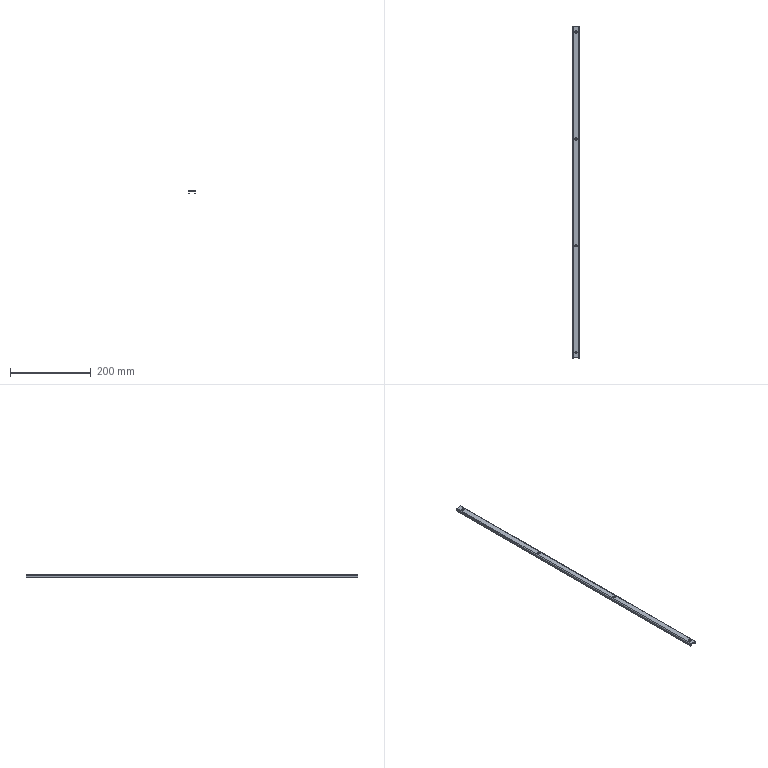Part | NX | features BREP 1 | 1 solid | 40 faces | box 17 x 820 x 7 mm | volume 42369 mm3 | plane 22 | cone 8 | cylinder 6 | torus 4 | commonest cylinder face diameters 0.2 x2 2 x2 4.2 x2
STEP:
#1=CARTESIAN_POINT('',(-2.7,395.,2.));
#2=VERTEX_POINT('',#1);
#3=CARTESIAN_POINT('',(2.7,395.,2.));
#4=VERTEX_POINT('',#3);
#5=CARTESIAN_POINT('',(0.,395.,2.));
#6=DIRECTION('',(0.,0.,1.));
#7=DIRECTION('',(1.,0.,0.));
#8=AXIS2_PLACEMENT_3D('',#5,#6,#7);
#9=CIRCLE('',#8,2.7);
#10=EDGE_CURVE('',#2,#4,#9,.T.);
#11=ORIENTED_EDGE('',*,*,#10,.T.);
#12=CARTESIAN_POINT('',(4.7,395.,0.));
#13=VERTEX_POINT('',#12);
#14=CARTESIAN_POINT('',(4.7,395.,0.));
#15=DIRECTION('',(0.7071,0.,-0.7071));
#16=VECTOR('',#15,1000.);
#17=LINE('',#14,#16);
#18=EDGE_CURVE('',#4,#13,#17,.T.);
#19=ORIENTED_EDGE('',*,*,#18,.T.);
#20=CARTESIAN_POINT('',(-4.7,395.,0.));
#21=VERTEX_POINT('',#20);
#22=CARTESIAN_POINT('',(0.,395.,0.));
#23=DIRECTION('',(0.,0.,-1.));
#24=DIRECTION('',(-1.,0.,0.));
#25=AXIS2_PLACEMENT_3D('',#22,#23,#24);
#26=CIRCLE('',#25,4.7);
#27=EDGE_CURVE('',#13,#21,#26,.T.);
#28=ORIENTED_EDGE('',*,*,#27,.T.);
#29=CARTESIAN_POINT('',(-4.7,395.,0.));
#30=DIRECTION('',(-0.7071,0.,-0.7071));
#31=VECTOR('',#30,1000.);
#32=LINE('',#29,#31);
#33=EDGE_CURVE('',#2,#21,#32,.T.);
#34=ORIENTED_EDGE('',*,*,#33,.F.);
#35=EDGE_LOOP('',(#11,#19,#28,#34));
#36=FACE_BOUND('',#35,.T.);
#37=CARTESIAN_POINT('',(0.,395.,0.));
#38=DIRECTION('',(0.,0.,-1.));
#39=DIRECTION('',(-1.,0.,0.));
#40=AXIS2_PLACEMENT_3D('',#37,#38,#39);
#41=CONICAL_SURFACE('',#40,4.7,0.7854);
#42=ADVANCED_FACE('',(#36),#41,.F.);
#43=CARTESIAN_POINT('',(-2.7,131.,2.));
#44=VERTEX_POINT('',#43);
#45=CARTESIAN_POINT('',(2.7,131.,2.));
#46=VERTEX_POINT('',#45);
#47=CARTESIAN_POINT('',(0.,131.,2.));
#48=DIRECTION('',(0.,0.,1.));
#49=DIRECTION('',(1.,0.,0.));
#50=AXIS2_PLACEMENT_3D('',#47,#48,#49);
#51=CIRCLE('',#50,2.7);
#52=EDGE_CURVE('',#44,#46,#51,.T.);
#53=ORIENTED_EDGE('',*,*,#52,.T.);
#54=CARTESIAN_POINT('',(4.7,131.,0.));
#55=VERTEX_POINT('',#54);
#56=CARTESIAN_POINT('',(4.7,131.,0.));
#57=DIRECTION('',(0.7071,0.,-0.7071));
#58=VECTOR('',#57,1000.);
#59=LINE('',#56,#58);
#60=EDGE_CURVE('',#46,#55,#59,.T.);
#61=ORIENTED_EDGE('',*,*,#60,.T.);
#62=CARTESIAN_POINT('',(-4.7,131.,0.));
#63=VERTEX_POINT('',#62);
#64=CARTESIAN_POINT('',(0.,131.,0.));
#65=DIRECTION('',(0.,0.,-1.));
#66=DIRECTION('',(-1.,0.,0.));
#67=AXIS2_PLACEMENT_3D('',#64,#65,#66);
#68=CIRCLE('',#67,4.7);
#69=EDGE_CURVE('',#55,#63,#68,.T.);
#70=ORIENTED_EDGE('',*,*,#69,.T.);
#71=CARTESIAN_POINT('',(-4.7,131.,0.));
#72=DIRECTION('',(-0.7071,0.,-0.7071));
#73=VECTOR('',#72,1000.);
#74=LINE('',#71,#73);
#75=EDGE_CURVE('',#44,#63,#74,.T.);
#76=ORIENTED_EDGE('',*,*,#75,.F.);
#77=EDGE_LOOP('',(#53,#61,#70,#76));
#78=FACE_BOUND('',#77,.T.);
#79=CARTESIAN_POINT('',(0.,131.,0.));
#80=DIRECTION('',(0.,0.,-1.));
#81=DIRECTION('',(-1.,0.,0.));
#82=AXIS2_PLACEMENT_3D('',#79,#80,#81);
#83=CONICAL_SURFACE('',#82,4.7,0.7854);
#84=ADVANCED_FACE('',(#78),#83,.F.);
#85=CARTESIAN_POINT('',(-2.7,-133.,2.));
#86=VERTEX_POINT('',#85);
#87=CARTESIAN_POINT('',(2.7,-133.,2.));
#88=VERTEX_POINT('',#87);
#89=CARTESIAN_POINT('',(0.,-133.,2.));
#90=DIRECTION('',(0.,0.,1.));
#91=DIRECTION('',(1.,0.,0.));
#92=AXIS2_PLACEMENT_3D('',#89,#90,#91);
#93=CIRCLE('',#92,2.7);
#94=EDGE_CURVE('',#86,#88,#93,.T.);
#95=ORIENTED_EDGE('',*,*,#94,.T.);
#96=CARTESIAN_POINT('',(4.7,-133.,0.));
#97=VERTEX_POINT('',#96);
#98=CARTESIAN_POINT('',(4.7,-133.,0.));
#99=DIRECTION('',(0.7071,0.,-0.7071));
#100=VECTOR('',#99,1000.);
#101=LINE('',#98,#100);
#102=EDGE_CURVE('',#88,#97,#101,.T.);
#103=ORIENTED_EDGE('',*,*,#102,.T.);
#104=CARTESIAN_POINT('',(-4.7,-133.,0.));
#105=VERTEX_POINT('',#104);
#106=CARTESIAN_POINT('',(0.,-133.,0.));
#107=DIRECTION('',(0.,0.,-1.));
#108=DIRECTION('',(-1.,0.,0.));
#109=AXIS2_PLACEMENT_3D('',#106,#107,#108);
#110=CIRCLE('',#109,4.7);
#111=EDGE_CURVE('',#97,#105,#110,.T.);
#112=ORIENTED_EDGE('',*,*,#111,.T.);
#113=CARTESIAN_POINT('',(-4.7,-133.,0.));
#114=DIRECTION('',(-0.7071,0.,-0.7071));
#115=VECTOR('',#114,1000.);
#116=LINE('',#113,#115);
#117=EDGE_CURVE('',#86,#105,#116,.T.);
#118=ORIENTED_EDGE('',*,*,#117,.F.);
#119=EDGE_LOOP('',(#95,#103,#112,#118));
#120=FACE_BOUND('',#119,.T.);
#121=CARTESIAN_POINT('',(0.,-133.,0.));
#122=DIRECTION('',(0.,0.,-1.));
#123=DIRECTION('',(-1.,0.,0.));
#124=AXIS2_PLACEMENT_3D('',#121,#122,#123);
#125=CONICAL_SURFACE('',#124,4.7,0.7854);
#126=ADVANCED_FACE('',(#120),#125,.F.);
#127=CARTESIAN_POINT('',(-2.7,-397.,2.));
#128=VERTEX_POINT('',#127);
#129=CARTESIAN_POINT('',(2.7,-397.,2.));
#130=VERTEX_POINT('',#129);
#131=CARTESIAN_POINT('',(0.,-397.,2.));
#132=DIRECTION('',(0.,0.,1.));
#133=DIRECTION('',(1.,0.,0.));
#134=AXIS2_PLACEMENT_3D('',#131,#132,#133);
#135=CIRCLE('',#134,2.7);
#136=EDGE_CURVE('',#128,#130,#135,.T.);
#137=ORIENTED_EDGE('',*,*,#136,.T.);
#138=CARTESIAN_POINT('',(4.7,-397.,0.));
#139=VERTEX_POINT('',#138);
#140=CARTESIAN_POINT('',(4.7,-397.,0.));
#141=DIRECTION('',(0.7071,0.,-0.7071));
#142=VECTOR('',#141,1000.);
#143=LINE('',#140,#142);
#144=EDGE_CURVE('',#130,#139,#143,.T.);
#145=ORIENTED_EDGE('',*,*,#144,.T.);
#146=CARTESIAN_POINT('',(-4.7,-397.,0.));
#147=VERTEX_POINT('',#146);
#148=CARTESIAN_POINT('',(0.,-397.,0.));
#149=DIRECTION('',(0.,0.,-1.));
#150=DIRECTION('',(-1.,0.,0.));
#151=AXIS2_PLACEMENT_3D('',#148,#149,#150);
#152=CIRCLE('',#151,4.7);
#153=EDGE_CURVE('',#139,#147,#152,.T.);
#154=ORIENTED_EDGE('',*,*,#153,.T.);
#155=CARTESIAN_POINT('',(-4.7,-397.,0.));
#156=DIRECTION('',(-0.7071,0.,-0.7071));
#157=VECTOR('',#156,1000.);
#158=LINE('',#155,#157);
#159=EDGE_CURVE('',#128,#147,#158,.T.);
#160=ORIENTED_EDGE('',*,*,#159,.F.);
#161=EDGE_LOOP('',(#137,#145,#154,#160));
#162=FACE_BOUND('',#161,.T.);
#163=CARTESIAN_POINT('',(0.,-397.,0.));
#164=DIRECTION('',(0.,0.,-1.));
#165=DIRECTION('',(-1.,0.,0.));
#166=AXIS2_PLACEMENT_3D('',#163,#164,#165);
#167=CONICAL_SURFACE('',#166,4.7,0.7854);
#168=ADVANCED_FACE('',(#162),#167,.F.);
#169=CARTESIAN_POINT('',(6.4,-410.,2.));
#170=VERTEX_POINT('',#169);
#171=CARTESIAN_POINT('',(-6.4,-410.,2.));
#172=VERTEX_POINT('',#171);
#173=CARTESIAN_POINT('',(-6.5,-410.,2.));
#174=DIRECTION('',(-1.,0.,0.));
#175=VECTOR('',#174,1000.);
#176=LINE('',#173,#175);
#177=EDGE_CURVE('',#170,#172,#176,.T.);
#178=ORIENTED_EDGE('',*,*,#177,.F.);
#179=CARTESIAN_POINT('',(6.4,410.,2.));
#180=VERTEX_POINT('',#179);
#181=CARTESIAN_POINT('',(6.4,410.,2.));
#182=DIRECTION('',(0.,-1.,0.));
#183=VECTOR('',#182,1000.);
#184=LINE('',#181,#183);
#185=EDGE_CURVE('',#180,#170,#184,.T.);
#186=ORIENTED_EDGE('',*,*,#185,.F.);
#187=CARTESIAN_POINT('',(-6.4,410.,2.));
#188=VERTEX_POINT('',#187);
#189=CARTESIAN_POINT('',(-6.5,410.,2.));
#190=DIRECTION('',(-1.,0.,0.));
#191=VECTOR('',#190,1000.);
#192=LINE('',#189,#191);
#193=EDGE_CURVE('',#180,#188,#192,.T.);
#194=ORIENTED_EDGE('',*,*,#193,.T.);
#195=CARTESIAN_POINT('',(-6.4,410.,2.));
#196=DIRECTION('',(0.,-1.,0.));
#197=VECTOR('',#196,1000.);
#198=LINE('',#195,#197);
#199=EDGE_CURVE('',#188,#172,#198,.T.);
#200=ORIENTED_EDGE('',*,*,#199,.T.);
#201=EDGE_LOOP('',(#178,#186,#194,#200));
#202=FACE_BOUND('',#201,.T.);
#203=ORIENTED_EDGE('',*,*,#10,.F.);
#204=CARTESIAN_POINT('',(0.,395.,2.));
#205=DIRECTION('',(0.,0.,1.));
#206=DIRECTION('',(1.,0.,0.));
#207=AXIS2_PLACEMENT_3D('',#204,#205,#206);
#208=CIRCLE('',#207,2.7);
#209=EDGE_CURVE('',#4,#2,#208,.T.);
#210=ORIENTED_EDGE('',*,*,#209,.F.);
#211=EDGE_LOOP('',(#203,#210));
#212=FACE_BOUND('',#211,.T.);
#213=ORIENTED_EDGE('',*,*,#136,.F.);
#214=CARTESIAN_POINT('',(0.,-397.,2.));
#215=DIRECTION('',(0.,0.,1.));
#216=DIRECTION('',(1.,0.,0.));
#217=AXIS2_PLACEMENT_3D('',#214,#215,#216);
#218=CIRCLE('',#217,2.7);
#219=EDGE_CURVE('',#130,#128,#218,.T.);
#220=ORIENTED_EDGE('',*,*,#219,.F.);
#221=EDGE_LOOP('',(#213,#220));
#222=FACE_BOUND('',#221,.T.);
#223=ORIENTED_EDGE('',*,*,#94,.F.);
#224=CARTESIAN_POINT('',(0.,-133.,2.));
#225=DIRECTION('',(0.,0.,1.));
#226=DIRECTION('',(1.,0.,0.));
#227=AXIS2_PLACEMENT_3D('',#224,#225,#226);
#228=CIRCLE('',#227,2.7);
#229=EDGE_CURVE('',#88,#86,#228,.T.);
#230=ORIENTED_EDGE('',*,*,#229,.F.);
#231=EDGE_LOOP('',(#223,#230));
#232=FACE_BOUND('',#231,.T.);
#233=ORIENTED_EDGE('',*,*,#52,.F.);
#234=CARTESIAN_POINT('',(0.,131.,2.));
#235=DIRECTION('',(0.,0.,1.));
#236=DIRECTION('',(1.,0.,0.));
#237=AXIS2_PLACEMENT_3D('',#234,#235,#236);
#238=CIRCLE('',#237,2.7);
#239=EDGE_CURVE('',#46,#44,#238,.T.);
#240=ORIENTED_EDGE('',*,*,#239,.F.);
#241=EDGE_LOOP('',(#233,#240));
#242=FACE_BOUND('',#241,.T.);
#243=CARTESIAN_POINT('',(-6.5,410.,2.));
#244=DIRECTION('',(0.,0.,1.));
#245=DIRECTION('',(1.,0.,0.));
#246=AXIS2_PLACEMENT_3D('',#243,#244,#245);
#247=PLANE('',#246);
#248=ADVANCED_FACE('',(#202,#212,#222,#232,#242),#247,.T.);
#249=CARTESIAN_POINT('',(7.5,410.,-0.1));
#250=VERTEX_POINT('',#249);
#251=CARTESIAN_POINT('',(8.5,410.,-0.1));
#252=VERTEX_POINT('',#251);
#253=CARTESIAN_POINT('',(6.5,410.,-0.1));
#254=DIRECTION('',(1.,0.,0.));
#255=VECTOR('',#254,1000.);
#256=LINE('',#253,#255);
#257=EDGE_CURVE('',#250,#252,#256,.T.);
#258=ORIENTED_EDGE('',*,*,#257,.F.);
#259=CARTESIAN_POINT('',(6.4,410.,1.));
#260=VERTEX_POINT('',#259);
#261=CARTESIAN_POINT('',(6.4,410.,-0.1));
#262=DIRECTION('',(0.,-1.,0.));
#263=DIRECTION('',(0.,0.,1.));
#264=AXIS2_PLACEMENT_3D('',#261,#262,#263);
#265=CIRCLE('',#264,1.1);
#266=EDGE_CURVE('',#250,#260,#265,.T.);
#267=ORIENTED_EDGE('',*,*,#266,.T.);
#268=CARTESIAN_POINT('',(6.4,410.,2.));
#269=DIRECTION('',(0.,0.,-1.));
#270=VECTOR('',#269,1000.);
#271=LINE('',#268,#270);
#272=EDGE_CURVE('',#180,#260,#271,.T.);
#273=ORIENTED_EDGE('',*,*,#272,.F.);
#274=CARTESIAN_POINT('',(6.4,410.,-0.1));
#275=DIRECTION('',(0.,-1.,0.));
#276=DIRECTION('',(1.,0.,0.));
#277=AXIS2_PLACEMENT_3D('',#274,#275,#276);
#278=CIRCLE('',#277,2.1);
#279=EDGE_CURVE('',#252,#180,#278,.T.);
#280=ORIENTED_EDGE('',*,*,#279,.F.);
#281=EDGE_LOOP('',(#258,#267,#273,#280));
#282=FACE_BOUND('',#281,.T.);
#283=CARTESIAN_POINT('',(6.5,410.,-0.1));
#284=DIRECTION('',(0.,1.,0.));
#285=DIRECTION('',(1.,0.,0.));
#286=AXIS2_PLACEMENT_3D('',#283,#284,#285);
#287=PLANE('',#286);
#288=ADVANCED_FACE('',(#282),#287,.T.);
#289=CARTESIAN_POINT('',(8.5,410.,-4.));
#290=VERTEX_POINT('',#289);
#291=CARTESIAN_POINT('',(8.5,410.,0.));
#292=DIRECTION('',(0.,0.,1.));
#293=VECTOR('',#292,1000.);
#294=LINE('',#291,#293);
#295=EDGE_CURVE('',#290,#252,#294,.T.);
#296=ORIENTED_EDGE('',*,*,#295,.F.);
#297=CARTESIAN_POINT('',(6.5,410.,-4.));
#298=VERTEX_POINT('',#297);
#299=CARTESIAN_POINT('',(6.4,410.,-4.));
#300=DIRECTION('',(-1.,0.,0.));
#301=VECTOR('',#300,1000.);
#302=LINE('',#299,#301);
#303=EDGE_CURVE('',#290,#298,#302,.T.);
#304=ORIENTED_EDGE('',*,*,#303,.T.);
#305=CARTESIAN_POINT('',(6.5,410.,-1.195));
#306=VERTEX_POINT('',#305);
#307=CARTESIAN_POINT('',(6.5,410.,0.));
#308=DIRECTION('',(0.,0.,1.));
#309=VECTOR('',#308,1000.);
#310=LINE('',#307,#309);
#311=EDGE_CURVE('',#298,#306,#310,.T.);
#312=ORIENTED_EDGE('',*,*,#311,.T.);
#313=CARTESIAN_POINT('',(6.4,410.,-0.1));
#314=DIRECTION('',(0.,-1.,0.));
#315=DIRECTION('',(0.,0.,1.));
#316=AXIS2_PLACEMENT_3D('',#313,#314,#315);
#317=CIRCLE('',#316,1.1);
#318=EDGE_CURVE('',#306,#250,#317,.T.);
#319=ORIENTED_EDGE('',*,*,#318,.T.);
#320=ORIENTED_EDGE('',*,*,#257,.T.);
#321=EDGE_LOOP('',(#296,#304,#312,#319,#320));
#322=FACE_BOUND('',#321,.T.);
#323=CARTESIAN_POINT('',(6.4,410.,2.));
#324=DIRECTION('',(0.,1.,0.));
#325=DIRECTION('',(1.,0.,0.));
#326=AXIS2_PLACEMENT_3D('',#323,#324,#325);
#327=PLANE('',#326);
#328=ADVANCED_FACE('',(#322),#327,.T.);
#329=CARTESIAN_POINT('',(6.4,-410.,1.));
#330=VERTEX_POINT('',#329);
#331=CARTESIAN_POINT('',(6.4,-410.,0.));
#332=DIRECTION('',(0.,0.,1.));
#333=VECTOR('',#332,1000.);
#334=LINE('',#331,#333);
#335=EDGE_CURVE('',#330,#170,#334,.T.);
#336=ORIENTED_EDGE('',*,*,#335,.F.);
#337=CARTESIAN_POINT('',(7.5,-410.,-0.1));
#338=VERTEX_POINT('',#337);
#339=CARTESIAN_POINT('',(6.4,-410.,-0.1));
#340=DIRECTION('',(0.,1.,0.));
#341=DIRECTION('',(0.,0.,-1.));
#342=AXIS2_PLACEMENT_3D('',#339,#340,#341);
#343=CIRCLE('',#342,1.1);
#344=EDGE_CURVE('',#330,#338,#343,.T.);
#345=ORIENTED_EDGE('',*,*,#344,.T.);
#346=CARTESIAN_POINT('',(8.5,-410.,-0.1));
#347=VERTEX_POINT('',#346);
#348=CARTESIAN_POINT('',(8.5,-410.,-0.1));
#349=DIRECTION('',(-1.,0.,0.));
#350=VECTOR('',#349,1000.);
#351=LINE('',#348,#350);
#352=EDGE_CURVE('',#347,#338,#351,.T.);
#353=ORIENTED_EDGE('',*,*,#352,.F.);
#354=CARTESIAN_POINT('',(6.4,-410.,-0.1));
#355=DIRECTION('',(0.,-1.,0.));
#356=DIRECTION('',(1.,0.,0.));
#357=AXIS2_PLACEMENT_3D('',#354,#355,#356);
#358=CIRCLE('',#357,2.1);
#359=EDGE_CURVE('',#347,#170,#358,.T.);
#360=ORIENTED_EDGE('',*,*,#359,.T.);
#361=EDGE_LOOP('',(#336,#345,#353,#360));
#362=FACE_BOUND('',#361,.T.);
#363=CARTESIAN_POINT('',(6.4,-410.,0.));
#364=DIRECTION('',(0.,-1.,0.));
#365=DIRECTION('',(0.,0.,-1.));
#366=AXIS2_PLACEMENT_3D('',#363,#364,#365);
#367=PLANE('',#366);
#368=ADVANCED_FACE('',(#362),#367,.T.);
#369=CARTESIAN_POINT('',(-6.4,-410.,1.));
#370=VERTEX_POINT('',#369);
#371=CARTESIAN_POINT('',(-6.4,-410.,2.));
#372=DIRECTION('',(0.,0.,-1.));
#373=VECTOR('',#372,1000.);
#374=LINE('',#371,#373);
#375=EDGE_CURVE('',#172,#370,#374,.T.);
#376=ORIENTED_EDGE('',*,*,#375,.T.);
#377=CARTESIAN_POINT('',(6.4,-410.,1.));
#378=DIRECTION('',(1.,0.,0.));
#379=VECTOR('',#378,1000.);
#380=LINE('',#377,#379);
#381=EDGE_CURVE('',#370,#330,#380,.T.);
#382=ORIENTED_EDGE('',*,*,#381,.T.);
#383=ORIENTED_EDGE('',*,*,#335,.T.);
#384=ORIENTED_EDGE('',*,*,#177,.T.);
#385=EDGE_LOOP('',(#376,#382,#383,#384));
#386=FACE_BOUND('',#385,.T.);
#387=CARTESIAN_POINT('',(8.5,-410.,-0.1));
#388=DIRECTION('',(0.,-1.,0.));
#389=DIRECTION('',(0.,0.,-1.));
#390=AXIS2_PLACEMENT_3D('',#387,#388,#389);
#391=PLANE('',#390);
#392=ADVANCED_FACE('',(#386),#391,.T.);
#393=CARTESIAN_POINT('',(-6.4,410.,1.));
#394=VERTEX_POINT('',#393);
#395=CARTESIAN_POINT('',(-6.4,410.,0.));
#396=DIRECTION('',(0.,0.,1.));
#397=VECTOR('',#396,1000.);
#398=LINE('',#395,#397);
#399=EDGE_CURVE('',#394,#188,#398,.T.);
#400=ORIENTED_EDGE('',*,*,#399,.F.);
#401=CARTESIAN_POINT('',(-7.5,410.,-0.1));
#402=VERTEX_POINT('',#401);
#403=CARTESIAN_POINT('',(-6.4,410.,-0.1));
#404=DIRECTION('',(0.,-1.,0.));
#405=DIRECTION('',(0.,0.,1.));
#406=AXIS2_PLACEMENT_3D('',#403,#404,#405);
#407=CIRCLE('',#406,1.1);
#408=EDGE_CURVE('',#394,#402,#407,.T.);
#409=ORIENTED_EDGE('',*,*,#408,.T.);
#410=CARTESIAN_POINT('',(-8.5,410.,-0.1));
#411=VERTEX_POINT('',#410);
#412=CARTESIAN_POINT('',(-8.5,410.,-0.1));
#413=DIRECTION('',(1.,0.,0.));
#414=VECTOR('',#413,1000.);
#415=LINE('',#412,#414);
#416=EDGE_CURVE('',#411,#402,#415,.T.);
#417=ORIENTED_EDGE('',*,*,#416,.F.);
#418=CARTESIAN_POINT('',(-6.4,410.,-0.1));
#419=DIRECTION('',(0.,-1.,0.));
#420=DIRECTION('',(1.,0.,0.));
#421=AXIS2_PLACEMENT_3D('',#418,#419,#420);
#422=CIRCLE('',#421,2.1);
#423=EDGE_CURVE('',#188,#411,#422,.T.);
#424=ORIENTED_EDGE('',*,*,#423,.F.);
#425=EDGE_LOOP('',(#400,#409,#417,#424));
#426=FACE_BOUND('',#425,.T.);
#427=CARTESIAN_POINT('',(-6.4,410.,0.));
#428=DIRECTION('',(0.,1.,0.));
#429=DIRECTION('',(1.,0.,0.));
#430=AXIS2_PLACEMENT_3D('',#427,#428,#429);
#431=PLANE('',#430);
#432=ADVANCED_FACE('',(#426),#431,.T.);
#433=ORIENTED_EDGE('',*,*,#272,.T.);
#434=CARTESIAN_POINT('',(-6.4,410.,1.));
#435=DIRECTION('',(-1.,0.,0.));
#436=VECTOR('',#435,1000.);
#437=LINE('',#434,#436);
#438=EDGE_CURVE('',#260,#394,#437,.T.);
#439=ORIENTED_EDGE('',*,*,#438,.T.);
#440=ORIENTED_EDGE('',*,*,#399,.T.);
#441=ORIENTED_EDGE('',*,*,#193,.F.);
#442=EDGE_LOOP('',(#433,#439,#440,#441));
#443=FACE_BOUND('',#442,.T.);
#444=CARTESIAN_POINT('',(-8.5,410.,-0.1));
#445=DIRECTION('',(0.,1.,0.));
#446=DIRECTION('',(1.,0.,0.));
#447=AXIS2_PLACEMENT_3D('',#444,#445,#446);
#448=PLANE('',#447);
#449=ADVANCED_FACE('',(#443),#448,.T.);
#450=CARTESIAN_POINT('',(-7.5,-410.,-0.1));
#451=VERTEX_POINT('',#450);
#452=CARTESIAN_POINT('',(-8.5,-410.,-0.1));
#453=VERTEX_POINT('',#452);
#454=CARTESIAN_POINT('',(-6.5,-410.,-0.1));
#455=DIRECTION('',(-1.,0.,0.));
#456=VECTOR('',#455,1000.);
#457=LINE('',#454,#456);
#458=EDGE_CURVE('',#451,#453,#457,.T.);
#459=ORIENTED_EDGE('',*,*,#458,.F.);
#460=CARTESIAN_POINT('',(-6.4,-410.,-0.1));
#461=DIRECTION('',(0.,1.,0.));
#462=DIRECTION('',(0.,0.,-1.));
#463=AXIS2_PLACEMENT_3D('',#460,#461,#462);
#464=CIRCLE('',#463,1.1);
#465=EDGE_CURVE('',#451,#370,#464,.T.);
#466=ORIENTED_EDGE('',*,*,#465,.T.);
#467=ORIENTED_EDGE('',*,*,#375,.F.);
#468=CARTESIAN_POINT('',(-6.4,-410.,-0.1));
#469=DIRECTION('',(0.,-1.,0.));
#470=DIRECTION('',(1.,0.,0.));
#471=AXIS2_PLACEMENT_3D('',#468,#469,#470);
#472=CIRCLE('',#471,2.1);
#473=EDGE_CURVE('',#172,#453,#472,.T.);
#474=ORIENTED_EDGE('',*,*,#473,.T.);
#475=EDGE_LOOP('',(#459,#466,#467,#474));
#476=FACE_BOUND('',#475,.T.);
#477=CARTESIAN_POINT('',(-6.5,-410.,-0.1));
#478=DIRECTION('',(0.,-1.,0.));
#479=DIRECTION('',(0.,0.,-1.));
#480=AXIS2_PLACEMENT_3D('',#477,#478,#479);
#481=PLANE('',#480);
#482=ADVANCED_FACE('',(#476),#481,.T.);
#483=CARTESIAN_POINT('',(-8.5,-410.,-4.));
#484=VERTEX_POINT('',#483);
#485=CARTESIAN_POINT('',(-8.5,-410.,0.));
#486=DIRECTION('',(0.,0.,-1.));
#487=VECTOR('',#486,1000.);
#488=LINE('',#485,#487);
#489=EDGE_CURVE('',#453,#484,#488,.T.);
#490=ORIENTED_EDGE('',*,*,#489,.T.);
#491=CARTESIAN_POINT('',(-6.5,-410.,-4.));
#492=VERTEX_POINT('',#491);
#493=CARTESIAN_POINT('',(-6.4,-410.,-4.));
#494=DIRECTION('',(1.,0.,0.));
#495=VECTOR('',#494,1000.);
#496=LINE('',#493,#495);
#497=EDGE_CURVE('',#484,#492,#496,.T.);
#498=ORIENTED_EDGE('',*,*,#497,.T.);
#499=CARTESIAN_POINT('',(-6.5,-410.,-1.195));
#500=VERTEX_POINT('',#499);
#501=CARTESIAN_POINT('',(-6.5,-410.,0.));
#502=DIRECTION('',(0.,0.,-1.));
#503=VECTOR('',#502,1000.);
#504=LINE('',#501,#503);
#505=EDGE_CURVE('',#500,#492,#504,.T.);
#506=ORIENTED_EDGE('',*,*,#505,.F.);
#507=CARTESIAN_POINT('',(-6.4,-410.,-0.1));
#508=DIRECTION('',(0.,1.,0.));
#509=DIRECTION('',(0.,0.,-1.));
#510=AXIS2_PLACEMENT_3D('',#507,#508,#509);
#511=CIRCLE('',#510,1.1);
#512=EDGE_CURVE('',#500,#451,#511,.T.);
#513=ORIENTED_EDGE('',*,*,#512,.T.);
#514=ORIENTED_EDGE('',*,*,#458,.T.);
#515=EDGE_LOOP('',(#490,#498,#506,#513,#514));
#516=FACE_BOUND('',#515,.T.);
#517=CARTESIAN_POINT('',(-6.4,-410.,2.));
#518=DIRECTION('',(0.,-1.,0.));
#519=DIRECTION('',(0.,0.,-1.));
#520=AXIS2_PLACEMENT_3D('',#517,#518,#519);
#521=PLANE('',#520);
#522=ADVANCED_FACE('',(#516),#521,.T.);
#523=CARTESIAN_POINT('',(-6.5,409.,-5.));
#524=VERTEX_POINT('',#523);
#525=CARTESIAN_POINT('',(-6.5,-409.,-5.));
#526=VERTEX_POINT('',#525);
#527=CARTESIAN_POINT('',(-6.5,410.,-5.));
#528=DIRECTION('',(0.,-1.,0.));
#529=VECTOR('',#528,1000.);
#530=LINE('',#527,#529);
#531=EDGE_CURVE('',#524,#526,#530,.T.);
#532=ORIENTED_EDGE('',*,*,#531,.F.);
#533=CARTESIAN_POINT('',(-6.5,410.,-4.));
#534=VERTEX_POINT('',#533);
#535=CARTESIAN_POINT('',(-6.5,409.,-5.));
#536=DIRECTION('',(0.,0.7071,0.7071));
#537=VECTOR('',#536,1000.);
#538=LINE('',#535,#537);
#539=EDGE_CURVE('',#524,#534,#538,.T.);
#540=ORIENTED_EDGE('',*,*,#539,.T.);
#541=CARTESIAN_POINT('',(-6.5,410.,-1.195));
#542=VERTEX_POINT('',#541);
#543=CARTESIAN_POINT('',(-6.5,410.,0.));
#544=DIRECTION('',(0.,0.,-1.));
#545=VECTOR('',#544,1000.);
#546=LINE('',#543,#545);
#547=EDGE_CURVE('',#542,#534,#546,.T.);
#548=ORIENTED_EDGE('',*,*,#547,.F.);
#549=CARTESIAN_POINT('',(-6.5,409.,-0.1));
#550=VERTEX_POINT('',#549);
#551=CARTESIAN_POINT('',(-6.5,410.,-1.195));
#552=CARTESIAN_POINT('',(-6.5,410.,-0.9262));
#553=CARTESIAN_POINT('',(-6.5,409.841,-0.5362));
#554=CARTESIAN_POINT('',(-6.5,409.369,-0.219));
#555=CARTESIAN_POINT('',(-6.5,409.163,-0.1517));
#556=CARTESIAN_POINT('',(-6.5,409.,-0.1));
#557=B_SPLINE_CURVE_WITH_KNOTS('',3,(#551,#552,#553,#554,#555,#556),.UNSPECIFIED.,.F.,.F.,(4,1,1,4),(0.,0.5,0.75,1.),.UNSPECIFIED.);
#558=EDGE_CURVE('',#542,#550,#557,.T.);
#559=ORIENTED_EDGE('',*,*,#558,.T.);
#560=CARTESIAN_POINT('',(-6.5,-409.,-0.1));
#561=VERTEX_POINT('',#560);
#562=CARTESIAN_POINT('',(-6.5,410.,-0.1));
#563=DIRECTION('',(0.,-1.,0.));
#564=VECTOR('',#563,1000.);
#565=LINE('',#562,#564);
#566=EDGE_CURVE('',#550,#561,#565,.T.);
#567=ORIENTED_EDGE('',*,*,#566,.T.);
#568=CARTESIAN_POINT('',(-6.5,-409.,-0.1));
#569=CARTESIAN_POINT('',(-6.5,-409.162,-0.1513));
#570=CARTESIAN_POINT('',(-6.5,-409.369,-0.2191));
#571=CARTESIAN_POINT('',(-6.5,-409.84,-0.5364));
#572=CARTESIAN_POINT('',(-6.5,-410.,-0.9248));
#573=CARTESIAN_POINT('',(-6.5,-410.,-1.195));
#574=B_SPLINE_CURVE_WITH_KNOTS('',3,(#568,#569,#570,#571,#572,#573),.UNSPECIFIED.,.F.,.F.,(4,1,1,4),(0.,0.25,0.5,1.),.UNSPECIFIED.);
#575=EDGE_CURVE('',#561,#500,#574,.T.);
#576=ORIENTED_EDGE('',*,*,#575,.T.);
#577=ORIENTED_EDGE('',*,*,#505,.T.);
#578=CARTESIAN_POINT('',(-6.5,-410.,-4.));
#579=DIRECTION('',(0.,0.7071,-0.7071));
#580=VECTOR('',#579,1000.);
#581=LINE('',#578,#580);
#582=EDGE_CURVE('',#492,#526,#581,.T.);
#583=ORIENTED_EDGE('',*,*,#582,.T.);
#584=EDGE_LOOP('',(#532,#540,#548,#559,#567,#576,#577,#583));
#585=FACE_BOUND('',#584,.T.);
#586=CARTESIAN_POINT('',(-6.5,410.,0.));
#587=DIRECTION('',(-1.,0.,0.));
#588=DIRECTION('',(0.,1.,0.));
#589=AXIS2_PLACEMENT_3D('',#586,#587,#588);
#590=PLANE('',#589);
#591=ADVANCED_FACE('',(#585),#590,.F.);
#592=CARTESIAN_POINT('',(-8.5,409.,-5.));
#593=VERTEX_POINT('',#592);
#594=CARTESIAN_POINT('',(-8.5,-409.,-5.));
#595=VERTEX_POINT('',#594);
#596=CARTESIAN_POINT('',(-8.5,410.,-5.));
#597=DIRECTION('',(0.,-1.,0.));
#598=VECTOR('',#597,1000.);
#599=LINE('',#596,#598);
#600=EDGE_CURVE('',#593,#595,#599,.T.);
#601=ORIENTED_EDGE('',*,*,#600,.F.);
#602=CARTESIAN_POINT('',(-8.5,409.,-5.));
#603=DIRECTION('',(1.,0.,0.));
#604=VECTOR('',#603,1000.);
#605=LINE('',#602,#604);
#606=EDGE_CURVE('',#593,#524,#605,.T.);
#607=ORIENTED_EDGE('',*,*,#606,.T.);
#608=ORIENTED_EDGE('',*,*,#531,.T.);
#609=CARTESIAN_POINT('',(-8.5,-409.,-5.));
#610=DIRECTION('',(-1.,0.,0.));
#611=VECTOR('',#610,1000.);
#612=LINE('',#609,#611);
#613=EDGE_CURVE('',#526,#595,#612,.T.);
#614=ORIENTED_EDGE('',*,*,#613,.T.);
#615=EDGE_LOOP('',(#601,#607,#608,#614));
#616=FACE_BOUND('',#615,.T.);
#617=CARTESIAN_POINT('',(-8.5,410.,-5.));
#618=DIRECTION('',(0.,0.,-1.));
#619=DIRECTION('',(-1.,0.,0.));
#620=AXIS2_PLACEMENT_3D('',#617,#618,#619);
#621=PLANE('',#620);
#622=ADVANCED_FACE('',(#616),#621,.T.);
#623=CARTESIAN_POINT('',(-8.5,410.,-4.));
#624=VERTEX_POINT('',#623);
#625=CARTESIAN_POINT('',(-8.5,410.,0.));
#626=DIRECTION('',(0.,0.,-1.));
#627=VECTOR('',#626,1000.);
#628=LINE('',#625,#627);
#629=EDGE_CURVE('',#411,#624,#628,.T.);
#630=ORIENTED_EDGE('',*,*,#629,.T.);
#631=CARTESIAN_POINT('',(-8.5,412.,-2.));
#632=DIRECTION('',(0.,-0.7071,-0.7071));
#633=VECTOR('',#632,1000.);
#634=LINE('',#631,#633);
#635=EDGE_CURVE('',#624,#593,#634,.T.);
#636=ORIENTED_EDGE('',*,*,#635,.T.);
#637=ORIENTED_EDGE('',*,*,#600,.T.);
#638=CARTESIAN_POINT('',(-8.5,-2.,-412.));
#639=DIRECTION('',(0.,-0.7071,0.7071));
#640=VECTOR('',#639,1000.);
#641=LINE('',#638,#640);
#642=EDGE_CURVE('',#595,#484,#641,.T.);
#643=ORIENTED_EDGE('',*,*,#642,.T.);
#644=ORIENTED_EDGE('',*,*,#489,.F.);
#645=CARTESIAN_POINT('',(-8.5,410.,-0.1));
#646=DIRECTION('',(0.,-1.,0.));
#647=VECTOR('',#646,1000.);
#648=LINE('',#645,#647);
#649=EDGE_CURVE('',#411,#453,#648,.T.);
#650=ORIENTED_EDGE('',*,*,#649,.F.);
#651=EDGE_LOOP('',(#630,#636,#637,#643,#644,#650));
#652=FACE_BOUND('',#651,.T.);
#653=CARTESIAN_POINT('',(-8.5,410.,0.));
#654=DIRECTION('',(-1.,0.,0.));
#655=DIRECTION('',(0.,1.,0.));
#656=AXIS2_PLACEMENT_3D('',#653,#654,#655);
#657=PLANE('',#656);
#658=ADVANCED_FACE('',(#652),#657,.T.);
#659=ORIENTED_EDGE('',*,*,#473,.F.);
#660=ORIENTED_EDGE('',*,*,#199,.F.);
#661=ORIENTED_EDGE('',*,*,#423,.T.);
#662=ORIENTED_EDGE('',*,*,#649,.T.);
#663=EDGE_LOOP('',(#659,#660,#661,#662));
#664=FACE_BOUND('',#663,.T.);
#665=CARTESIAN_POINT('',(-6.4,410.,-0.1));
#666=DIRECTION('',(0.,-1.,0.));
#667=DIRECTION('',(0.,0.,-1.));
#668=AXIS2_PLACEMENT_3D('',#665,#666,#667);
#669=CYLINDRICAL_SURFACE('',#668,2.1);
#670=ADVANCED_FACE('',(#664),#669,.T.);
#671=ORIENTED_EDGE('',*,*,#359,.F.);
#672=CARTESIAN_POINT('',(8.5,410.,-0.1));
#673=DIRECTION('',(0.,-1.,0.));
#674=VECTOR('',#673,1000.);
#675=LINE('',#672,#674);
#676=EDGE_CURVE('',#252,#347,#675,.T.);
#677=ORIENTED_EDGE('',*,*,#676,.F.);
#678=ORIENTED_EDGE('',*,*,#279,.T.);
#679=ORIENTED_EDGE('',*,*,#185,.T.);
#680=EDGE_LOOP('',(#671,#677,#678,#679));
#681=FACE_BOUND('',#680,.T.);
#682=CARTESIAN_POINT('',(6.4,410.,-0.1));
#683=DIRECTION('',(0.,-1.,0.));
#684=DIRECTION('',(0.,0.,-1.));
#685=AXIS2_PLACEMENT_3D('',#682,#683,#684);
#686=CYLINDRICAL_SURFACE('',#685,2.1);
#687=ADVANCED_FACE('',(#681),#686,.T.);
#688=CARTESIAN_POINT('',(8.5,409.,-5.));
#689=VERTEX_POINT('',#688);
#690=CARTESIAN_POINT('',(8.5,-409.,-5.));
#691=VERTEX_POINT('',#690);
#692=CARTESIAN_POINT('',(8.5,410.,-5.));
#693=DIRECTION('',(0.,-1.,0.));
#694=VECTOR('',#693,1000.);
#695=LINE('',#692,#694);
#696=EDGE_CURVE('',#689,#691,#695,.T.);
#697=ORIENTED_EDGE('',*,*,#696,.F.);
#698=CARTESIAN_POINT('',(8.5,412.,-2.));
#699=DIRECTION('',(0.,0.7071,0.7071));
#700=VECTOR('',#699,1000.);
#701=LINE('',#698,#700);
#702=EDGE_CURVE('',#689,#290,#701,.T.);
#703=ORIENTED_EDGE('',*,*,#702,.T.);
#704=ORIENTED_EDGE('',*,*,#295,.T.);
#705=ORIENTED_EDGE('',*,*,#676,.T.);
#706=CARTESIAN_POINT('',(8.5,-410.,-4.));
#707=VERTEX_POINT('',#706);
#708=CARTESIAN_POINT('',(8.5,-410.,0.));
#709=DIRECTION('',(0.,0.,1.));
#710=VECTOR('',#709,1000.);
#711=LINE('',#708,#710);
#712=EDGE_CURVE('',#707,#347,#711,.T.);
#713=ORIENTED_EDGE('',*,*,#712,.F.);
#714=CARTESIAN_POINT('',(8.5,-2.,-412.));
#715=DIRECTION('',(0.,0.7071,-0.7071));
#716=VECTOR('',#715,1000.);
#717=LINE('',#714,#716);
#718=EDGE_CURVE('',#707,#691,#717,.T.);
#719=ORIENTED_EDGE('',*,*,#718,.T.);
#720=EDGE_LOOP('',(#697,#703,#704,#705,#713,#719));
#721=FACE_BOUND('',#720,.T.);
#722=CARTESIAN_POINT('',(8.5,410.,0.));
#723=DIRECTION('',(1.,0.,0.));
#724=DIRECTION('',(0.,1.,0.));
#725=AXIS2_PLACEMENT_3D('',#722,#723,#724);
#726=PLANE('',#725);
#727=ADVANCED_FACE('',(#721),#726,.T.);
#728=CARTESIAN_POINT('',(6.5,409.,-5.));
#729=VERTEX_POINT('',#728);
#730=CARTESIAN_POINT('',(6.5,-409.,-5.));
#731=VERTEX_POINT('',#730);
#732=CARTESIAN_POINT('',(6.5,410.,-5.));
#733=DIRECTION('',(0.,-1.,0.));
#734=VECTOR('',#733,1000.);
#735=LINE('',#732,#734);
#736=EDGE_CURVE('',#729,#731,#735,.T.);
#737=ORIENTED_EDGE('',*,*,#736,.F.);
#738=CARTESIAN_POINT('',(6.5,409.,-5.));
#739=DIRECTION('',(1.,0.,0.));
#740=VECTOR('',#739,1000.);
#741=LINE('',#738,#740);
#742=EDGE_CURVE('',#729,#689,#741,.T.);
#743=ORIENTED_EDGE('',*,*,#742,.T.);
#744=ORIENTED_EDGE('',*,*,#696,.T.);
#745=CARTESIAN_POINT('',(6.5,-409.,-5.));
#746=DIRECTION('',(-1.,0.,0.));
#747=VECTOR('',#746,1000.);
#748=LINE('',#745,#747);
#749=EDGE_CURVE('',#691,#731,#748,.T.);
#750=ORIENTED_EDGE('',*,*,#749,.T.);
#751=EDGE_LOOP('',(#737,#743,#744,#750));
#752=FACE_BOUND('',#751,.T.);
#753=CARTESIAN_POINT('',(6.5,410.,-5.));
#754=DIRECTION('',(0.,0.,-1.));
#755=DIRECTION('',(0.,-1.,0.));
#756=AXIS2_PLACEMENT_3D('',#753,#754,#755);
#757=PLANE('',#756);
#758=ADVANCED_FACE('',(#752),#757,.T.);
#759=ORIENTED_EDGE('',*,*,#311,.F.);
#760=CARTESIAN_POINT('',(6.5,409.,-5.));
#761=DIRECTION('',(0.,-0.7071,-0.7071));
#762=VECTOR('',#761,1000.);
#763=LINE('',#760,#762);
#764=EDGE_CURVE('',#298,#729,#763,.T.);
#765=ORIENTED_EDGE('',*,*,#764,.T.);
#766=ORIENTED_EDGE('',*,*,#736,.T.);
#767=CARTESIAN_POINT('',(6.5,-410.,-4.));
#768=VERTEX_POINT('',#767);
#769=CARTESIAN_POINT('',(6.5,-410.,-4.));
#770=DIRECTION('',(0.,-0.7071,0.7071));
#771=VECTOR('',#770,1000.);
#772=LINE('',#769,#771);
#773=EDGE_CURVE('',#731,#768,#772,.T.);
#774=ORIENTED_EDGE('',*,*,#773,.T.);
#775=CARTESIAN_POINT('',(6.5,-410.,-1.195));
#776=VERTEX_POINT('',#775);
#777=CARTESIAN_POINT('',(6.5,-410.,0.));
#778=DIRECTION('',(0.,0.,1.));
#779=VECTOR('',#778,1000.);
#780=LINE('',#777,#779);
#781=EDGE_CURVE('',#768,#776,#780,.T.);
#782=ORIENTED_EDGE('',*,*,#781,.T.);
#783=CARTESIAN_POINT('',(6.5,-409.,-0.1));
#784=VERTEX_POINT('',#783);
#785=CARTESIAN_POINT('',(6.5,-410.,-1.195));
#786=CARTESIAN_POINT('',(6.5,-410.,-0.9262));
#787=CARTESIAN_POINT('',(6.5,-409.841,-0.5362));
#788=CARTESIAN_POINT('',(6.5,-409.369,-0.219));
#789=CARTESIAN_POINT('',(6.5,-409.163,-0.1517));
#790=CARTESIAN_POINT('',(6.5,-409.,-0.1));
#791=B_SPLINE_CURVE_WITH_KNOTS('',3,(#785,#786,#787,#788,#789,#790),.UNSPECIFIED.,.F.,.F.,(4,1,1,4),(0.,0.5,0.75,1.),.UNSPECIFIED.);
#792=EDGE_CURVE('',#776,#784,#791,.T.);
#793=ORIENTED_EDGE('',*,*,#792,.T.);
#794=CARTESIAN_POINT('',(6.5,409.,-0.1));
#795=VERTEX_POINT('',#794);
#796=CARTESIAN_POINT('',(6.5,410.,-0.1));
#797=DIRECTION('',(0.,-1.,0.));
#798=VECTOR('',#797,1000.);
#799=LINE('',#796,#798);
#800=EDGE_CURVE('',#795,#784,#799,.T.);
#801=ORIENTED_EDGE('',*,*,#800,.F.);
#802=CARTESIAN_POINT('',(6.5,409.,-0.1));
#803=CARTESIAN_POINT('',(6.5,409.162,-0.1513));
#804=CARTESIAN_POINT('',(6.5,409.369,-0.2191));
#805=CARTESIAN_POINT('',(6.5,409.84,-0.5364));
#806=CARTESIAN_POINT('',(6.5,410.,-0.9248));
#807=CARTESIAN_POINT('',(6.5,410.,-1.195));
#808=B_SPLINE_CURVE_WITH_KNOTS('',3,(#802,#803,#804,#805,#806,#807),.UNSPECIFIED.,.F.,.F.,(4,1,1,4),(0.,0.25,0.5,1.),.UNSPECIFIED.);
#809=EDGE_CURVE('',#795,#306,#808,.T.);
#810=ORIENTED_EDGE('',*,*,#809,.T.);
#811=EDGE_LOOP('',(#759,#765,#766,#774,#782,#793,#801,#810));
#812=FACE_BOUND('',#811,.T.);
#813=CARTESIAN_POINT('',(6.5,410.,0.));
#814=DIRECTION('',(1.,0.,0.));
#815=DIRECTION('',(0.,1.,0.));
#816=AXIS2_PLACEMENT_3D('',#813,#814,#815);
#817=PLANE('',#816);
#818=ADVANCED_FACE('',(#812),#817,.F.);
#819=CARTESIAN_POINT('',(6.4,409.,0.));
#820=VERTEX_POINT('',#819);
#821=CARTESIAN_POINT('',(6.4,-409.,0.));
#822=VERTEX_POINT('',#821);
#823=CARTESIAN_POINT('',(6.4,410.,0.));
#824=DIRECTION('',(0.,-1.,0.));
#825=VECTOR('',#824,1000.);
#826=LINE('',#823,#825);
#827=EDGE_CURVE('',#820,#822,#826,.T.);
#828=ORIENTED_EDGE('',*,*,#827,.F.);
#829=CARTESIAN_POINT('',(6.4,409.,-0.1));
#830=DIRECTION('',(0.,1.,0.));
#831=DIRECTION('',(0.,0.,1.));
#832=AXIS2_PLACEMENT_3D('',#829,#830,#831);
#833=CIRCLE('',#832,0.1);
#834=EDGE_CURVE('',#820,#795,#833,.T.);
#835=ORIENTED_EDGE('',*,*,#834,.T.);
#836=ORIENTED_EDGE('',*,*,#800,.T.);
#837=CARTESIAN_POINT('',(6.4,-409.,-0.1));
#838=DIRECTION('',(0.,-1.,0.));
#839=DIRECTION('',(0.,0.,-1.));
#840=AXIS2_PLACEMENT_3D('',#837,#838,#839);
#841=CIRCLE('',#840,0.1);
#842=EDGE_CURVE('',#784,#822,#841,.T.);
#843=ORIENTED_EDGE('',*,*,#842,.T.);
#844=EDGE_LOOP('',(#828,#835,#836,#843));
#845=FACE_BOUND('',#844,.T.);
#846=CARTESIAN_POINT('',(6.4,410.,-0.1));
#847=DIRECTION('',(0.,-1.,0.));
#848=DIRECTION('',(0.,0.,-1.));
#849=AXIS2_PLACEMENT_3D('',#846,#847,#848);
#850=CYLINDRICAL_SURFACE('',#849,0.1);
#851=ADVANCED_FACE('',(#845),#850,.F.);
#852=CARTESIAN_POINT('',(-6.4,409.,0.));
#853=VERTEX_POINT('',#852);
#854=CARTESIAN_POINT('',(-6.4,-409.,0.));
#855=VERTEX_POINT('',#854);
#856=CARTESIAN_POINT('',(-6.4,410.,0.));
#857=DIRECTION('',(0.,-1.,0.));
#858=VECTOR('',#857,1000.);
#859=LINE('',#856,#858);
#860=EDGE_CURVE('',#853,#855,#859,.T.);
#861=ORIENTED_EDGE('',*,*,#860,.F.);
#862=CARTESIAN_POINT('',(6.4,409.,0.));
#863=DIRECTION('',(1.,0.,0.));
#864=VECTOR('',#863,1000.);
#865=LINE('',#862,#864);
#866=EDGE_CURVE('',#853,#820,#865,.T.);
#867=ORIENTED_EDGE('',*,*,#866,.T.);
#868=ORIENTED_EDGE('',*,*,#827,.T.);
#869=CARTESIAN_POINT('',(-6.4,-409.,0.));
#870=DIRECTION('',(-1.,0.,0.));
#871=VECTOR('',#870,1000.);
#872=LINE('',#869,#871);
#873=EDGE_CURVE('',#822,#855,#872,.T.);
#874=ORIENTED_EDGE('',*,*,#873,.T.);
#875=EDGE_LOOP('',(#861,#867,#868,#874));
#876=FACE_BOUND('',#875,.T.);
#877=CARTESIAN_POINT('',(0.,395.,0.));
#878=DIRECTION('',(0.,0.,-1.));
#879=DIRECTION('',(-1.,0.,0.));
#880=AXIS2_PLACEMENT_3D('',#877,#878,#879);
#881=CIRCLE('',#880,4.7);
#882=EDGE_CURVE('',#21,#13,#881,.T.);
#883=ORIENTED_EDGE('',*,*,#882,.F.);
#884=ORIENTED_EDGE('',*,*,#27,.F.);
#885=EDGE_LOOP('',(#883,#884));
#886=FACE_BOUND('',#885,.T.);
#887=CARTESIAN_POINT('',(0.,131.,0.));
#888=DIRECTION('',(0.,0.,-1.));
#889=DIRECTION('',(-1.,0.,0.));
#890=AXIS2_PLACEMENT_3D('',#887,#888,#889);
#891=CIRCLE('',#890,4.7);
#892=EDGE_CURVE('',#63,#55,#891,.T.);
#893=ORIENTED_EDGE('',*,*,#892,.F.);
#894=ORIENTED_EDGE('',*,*,#69,.F.);
#895=EDGE_LOOP('',(#893,#894));
#896=FACE_BOUND('',#895,.T.);
#897=CARTESIAN_POINT('',(0.,-133.,0.));
#898=DIRECTION('',(0.,0.,-1.));
#899=DIRECTION('',(-1.,0.,0.));
#900=AXIS2_PLACEMENT_3D('',#897,#898,#899);
#901=CIRCLE('',#900,4.7);
#902=EDGE_CURVE('',#105,#97,#901,.T.);
#903=ORIENTED_EDGE('',*,*,#902,.F.);
#904=ORIENTED_EDGE('',*,*,#111,.F.);
#905=EDGE_LOOP('',(#903,#904));
#906=FACE_BOUND('',#905,.T.);
#907=CARTESIAN_POINT('',(0.,-397.,0.));
#908=DIRECTION('',(0.,0.,-1.));
#909=DIRECTION('',(-1.,0.,0.));
#910=AXIS2_PLACEMENT_3D('',#907,#908,#909);
#911=CIRCLE('',#910,4.7);
#912=EDGE_CURVE('',#147,#139,#911,.T.);
#913=ORIENTED_EDGE('',*,*,#912,.F.);
#914=ORIENTED_EDGE('',*,*,#153,.F.);
#915=EDGE_LOOP('',(#913,#914));
#916=FACE_BOUND('',#915,.T.);
#917=CARTESIAN_POINT('',(-6.5,410.,0.));
#918=DIRECTION('',(0.,0.,1.));
#919=DIRECTION('',(1.,0.,0.));
#920=AXIS2_PLACEMENT_3D('',#917,#918,#919);
#921=PLANE('',#920);
#922=ADVANCED_FACE('',(#876,#886,#896,#906,#916),#921,.F.);
#923=ORIENTED_EDGE('',*,*,#566,.F.);
#924=CARTESIAN_POINT('',(-6.4,409.,-0.1));
#925=DIRECTION('',(0.,1.,0.));
#926=DIRECTION('',(0.,0.,1.));
#927=AXIS2_PLACEMENT_3D('',#924,#925,#926);
#928=CIRCLE('',#927,0.1);
#929=EDGE_CURVE('',#550,#853,#928,.T.);
#930=ORIENTED_EDGE('',*,*,#929,.T.);
#931=ORIENTED_EDGE('',*,*,#860,.T.);
#932=CARTESIAN_POINT('',(-6.4,-409.,-0.1));
#933=DIRECTION('',(0.,-1.,0.));
#934=DIRECTION('',(0.,0.,-1.));
#935=AXIS2_PLACEMENT_3D('',#932,#933,#934);
#936=CIRCLE('',#935,0.1);
#937=EDGE_CURVE('',#855,#561,#936,.T.);
#938=ORIENTED_EDGE('',*,*,#937,.T.);
#939=EDGE_LOOP('',(#923,#930,#931,#938));
#940=FACE_BOUND('',#939,.T.);
#941=CARTESIAN_POINT('',(-6.4,410.,-0.1));
#942=DIRECTION('',(0.,-1.,0.));
#943=DIRECTION('',(0.,0.,-1.));
#944=AXIS2_PLACEMENT_3D('',#941,#942,#943);
#945=CYLINDRICAL_SURFACE('',#944,0.1);
#946=ADVANCED_FACE('',(#940),#945,.F.);
#947=ORIENTED_EDGE('',*,*,#547,.T.);
#948=CARTESIAN_POINT('',(-6.4,410.,-4.));
#949=DIRECTION('',(-1.,0.,0.));
#950=VECTOR('',#949,1000.);
#951=LINE('',#948,#950);
#952=EDGE_CURVE('',#534,#624,#951,.T.);
#953=ORIENTED_EDGE('',*,*,#952,.T.);
#954=ORIENTED_EDGE('',*,*,#629,.F.);
#955=ORIENTED_EDGE('',*,*,#416,.T.);
#956=CARTESIAN_POINT('',(-6.4,410.,-0.1));
#957=DIRECTION('',(0.,-1.,0.));
#958=DIRECTION('',(0.,0.,1.));
#959=AXIS2_PLACEMENT_3D('',#956,#957,#958);
#960=CIRCLE('',#959,1.1);
#961=EDGE_CURVE('',#402,#542,#960,.T.);
#962=ORIENTED_EDGE('',*,*,#961,.T.);
#963=EDGE_LOOP('',(#947,#953,#954,#955,#962));
#964=FACE_BOUND('',#963,.T.);
#965=CARTESIAN_POINT('',(-6.4,410.,-0.1));
#966=DIRECTION('',(0.,1.,0.));
#967=DIRECTION('',(1.,0.,0.));
#968=AXIS2_PLACEMENT_3D('',#965,#966,#967);
#969=PLANE('',#968);
#970=ADVANCED_FACE('',(#964),#969,.T.);
#971=ORIENTED_EDGE('',*,*,#781,.F.);
#972=CARTESIAN_POINT('',(8.5,-410.,-4.));
#973=DIRECTION('',(1.,0.,0.));
#974=VECTOR('',#973,1000.);
#975=LINE('',#972,#974);
#976=EDGE_CURVE('',#768,#707,#975,.T.);
#977=ORIENTED_EDGE('',*,*,#976,.T.);
#978=ORIENTED_EDGE('',*,*,#712,.T.);
#979=ORIENTED_EDGE('',*,*,#352,.T.);
#980=CARTESIAN_POINT('',(6.4,-410.,-0.1));
#981=DIRECTION('',(0.,1.,0.));
#982=DIRECTION('',(0.,0.,-1.));
#983=AXIS2_PLACEMENT_3D('',#980,#981,#982);
#984=CIRCLE('',#983,1.1);
#985=EDGE_CURVE('',#338,#776,#984,.T.);
#986=ORIENTED_EDGE('',*,*,#985,.T.);
#987=EDGE_LOOP('',(#971,#977,#978,#979,#986));
#988=FACE_BOUND('',#987,.T.);
#989=CARTESIAN_POINT('',(-6.4,-410.,-0.1));
#990=DIRECTION('',(0.,1.,0.));
#991=DIRECTION('',(1.,0.,0.));
#992=AXIS2_PLACEMENT_3D('',#989,#990,#991);
#993=PLANE('',#992);
#994=ADVANCED_FACE('',(#988),#993,.F.);
#995=ORIENTED_EDGE('',*,*,#144,.F.);
#996=ORIENTED_EDGE('',*,*,#219,.T.);
#997=ORIENTED_EDGE('',*,*,#159,.T.);
#998=ORIENTED_EDGE('',*,*,#912,.T.);
#999=EDGE_LOOP('',(#995,#996,#997,#998));
#1000=FACE_BOUND('',#999,.T.);
#1001=CARTESIAN_POINT('',(0.,-397.,0.));
#1002=DIRECTION('',(0.,0.,-1.));
#1003=DIRECTION('',(-1.,0.,0.));
#1004=AXIS2_PLACEMENT_3D('',#1001,#1002,#1003);
#1005=CONICAL_SURFACE('',#1004,4.7,0.7854);
#1006=ADVANCED_FACE('',(#1000),#1005,.F.);
#1007=ORIENTED_EDGE('',*,*,#102,.F.);
#1008=ORIENTED_EDGE('',*,*,#229,.T.);
#1009=ORIENTED_EDGE('',*,*,#117,.T.);
#1010=ORIENTED_EDGE('',*,*,#902,.T.);
#1011=EDGE_LOOP('',(#1007,#1008,#1009,#1010));
#1012=FACE_BOUND('',#1011,.T.);
#1013=CARTESIAN_POINT('',(0.,-133.,0.));
#1014=DIRECTION('',(0.,0.,-1.));
#1015=DIRECTION('',(-1.,0.,0.));
#1016=AXIS2_PLACEMENT_3D('',#1013,#1014,#1015);
#1017=CONICAL_SURFACE('',#1016,4.7,0.7854);
#1018=ADVANCED_FACE('',(#1012),#1017,.F.);
#1019=ORIENTED_EDGE('',*,*,#60,.F.);
#1020=ORIENTED_EDGE('',*,*,#239,.T.);
#1021=ORIENTED_EDGE('',*,*,#75,.T.);
#1022=ORIENTED_EDGE('',*,*,#892,.T.);
#1023=EDGE_LOOP('',(#1019,#1020,#1021,#1022));
#1024=FACE_BOUND('',#1023,.T.);
#1025=CARTESIAN_POINT('',(0.,131.,0.));
#1026=DIRECTION('',(0.,0.,-1.));
#1027=DIRECTION('',(-1.,0.,0.));
#1028=AXIS2_PLACEMENT_3D('',#1025,#1026,#1027);
#1029=CONICAL_SURFACE('',#1028,4.7,0.7854);
#1030=ADVANCED_FACE('',(#1024),#1029,.F.);
#1031=ORIENTED_EDGE('',*,*,#18,.F.);
#1032=ORIENTED_EDGE('',*,*,#209,.T.);
#1033=ORIENTED_EDGE('',*,*,#33,.T.);
#1034=ORIENTED_EDGE('',*,*,#882,.T.);
#1035=EDGE_LOOP('',(#1031,#1032,#1033,#1034));
#1036=FACE_BOUND('',#1035,.T.);
#1037=CARTESIAN_POINT('',(0.,395.,0.));
#1038=DIRECTION('',(0.,0.,-1.));
#1039=DIRECTION('',(-1.,0.,0.));
#1040=AXIS2_PLACEMENT_3D('',#1037,#1038,#1039);
#1041=CONICAL_SURFACE('',#1040,4.7,0.7854);
#1042=ADVANCED_FACE('',(#1036),#1041,.F.);
#1043=ORIENTED_EDGE('',*,*,#961,.F.);
#1044=ORIENTED_EDGE('',*,*,#408,.F.);
#1045=CARTESIAN_POINT('',(-6.4,409.,1.));
#1046=DIRECTION('',(1.,0.,0.));
#1047=DIRECTION('',(0.,0.,-1.));
#1048=AXIS2_PLACEMENT_3D('',#1045,#1046,#1047);
#1049=CIRCLE('',#1048,1.);
#1050=EDGE_CURVE('',#853,#394,#1049,.T.);
#1051=ORIENTED_EDGE('',*,*,#1050,.F.);
#1052=ORIENTED_EDGE('',*,*,#929,.F.);
#1053=ORIENTED_EDGE('',*,*,#558,.F.);
#1054=EDGE_LOOP('',(#1043,#1044,#1051,#1052,#1053));
#1055=FACE_BOUND('',#1054,.T.);
#1056=CARTESIAN_POINT('',(-6.4,409.,-0.1));
#1057=DIRECTION('',(0.,1.,0.));
#1058=DIRECTION('',(0.,0.,1.));
#1059=AXIS2_PLACEMENT_3D('',#1056,#1057,#1058);
#1060=TOROIDAL_SURFACE('',#1059,1.1,1.);
#1061=ADVANCED_FACE('',(#1055),#1060,.T.);
#1062=ORIENTED_EDGE('',*,*,#1050,.T.);
#1063=ORIENTED_EDGE('',*,*,#438,.F.);
#1064=CARTESIAN_POINT('',(6.4,409.,1.));
#1065=DIRECTION('',(1.,0.,0.));
#1066=DIRECTION('',(0.,0.,-1.));
#1067=AXIS2_PLACEMENT_3D('',#1064,#1065,#1066);
#1068=CIRCLE('',#1067,1.);
#1069=EDGE_CURVE('',#820,#260,#1068,.T.);
#1070=ORIENTED_EDGE('',*,*,#1069,.F.);
#1071=ORIENTED_EDGE('',*,*,#866,.F.);
#1072=EDGE_LOOP('',(#1062,#1063,#1070,#1071));
#1073=FACE_BOUND('',#1072,.T.);
#1074=CARTESIAN_POINT('',(-8.5,409.,1.));
#1075=DIRECTION('',(1.,0.,0.));
#1076=DIRECTION('',(0.,0.,-1.));
#1077=AXIS2_PLACEMENT_3D('',#1074,#1075,#1076);
#1078=CYLINDRICAL_SURFACE('',#1077,1.);
#1079=ADVANCED_FACE('',(#1073),#1078,.T.);
#1080=ORIENTED_EDGE('',*,*,#809,.F.);
#1081=ORIENTED_EDGE('',*,*,#834,.F.);
#1082=ORIENTED_EDGE('',*,*,#1069,.T.);
#1083=ORIENTED_EDGE('',*,*,#266,.F.);
#1084=ORIENTED_EDGE('',*,*,#318,.F.);
#1085=EDGE_LOOP('',(#1080,#1081,#1082,#1083,#1084));
#1086=FACE_BOUND('',#1085,.T.);
#1087=CARTESIAN_POINT('',(6.4,409.,-0.1));
#1088=DIRECTION('',(0.,1.,0.));
#1089=DIRECTION('',(0.,0.,1.));
#1090=AXIS2_PLACEMENT_3D('',#1087,#1088,#1089);
#1091=TOROIDAL_SURFACE('',#1090,1.1,1.);
#1092=ADVANCED_FACE('',(#1086),#1091,.T.);
#1093=ORIENTED_EDGE('',*,*,#575,.F.);
#1094=ORIENTED_EDGE('',*,*,#937,.F.);
#1095=CARTESIAN_POINT('',(-6.4,-409.,1.));
#1096=DIRECTION('',(1.,0.,0.));
#1097=DIRECTION('',(0.,0.,-1.));
#1098=AXIS2_PLACEMENT_3D('',#1095,#1096,#1097);
#1099=CIRCLE('',#1098,1.);
#1100=EDGE_CURVE('',#370,#855,#1099,.T.);
#1101=ORIENTED_EDGE('',*,*,#1100,.F.);
#1102=ORIENTED_EDGE('',*,*,#465,.F.);
#1103=ORIENTED_EDGE('',*,*,#512,.F.);
#1104=EDGE_LOOP('',(#1093,#1094,#1101,#1102,#1103));
#1105=FACE_BOUND('',#1104,.T.);
#1106=CARTESIAN_POINT('',(-6.4,-409.,-0.1));
#1107=DIRECTION('',(0.,-1.,0.));
#1108=DIRECTION('',(0.,0.,-1.));
#1109=AXIS2_PLACEMENT_3D('',#1106,#1107,#1108);
#1110=TOROIDAL_SURFACE('',#1109,1.1,1.);
#1111=ADVANCED_FACE('',(#1105),#1110,.T.);
#1112=ORIENTED_EDGE('',*,*,#1100,.T.);
#1113=ORIENTED_EDGE('',*,*,#873,.F.);
#1114=CARTESIAN_POINT('',(6.4,-409.,1.));
#1115=DIRECTION('',(1.,0.,0.));
#1116=DIRECTION('',(0.,0.,-1.));
#1117=AXIS2_PLACEMENT_3D('',#1114,#1115,#1116);
#1118=CIRCLE('',#1117,1.);
#1119=EDGE_CURVE('',#330,#822,#1118,.T.);
#1120=ORIENTED_EDGE('',*,*,#1119,.F.);
#1121=ORIENTED_EDGE('',*,*,#381,.F.);
#1122=EDGE_LOOP('',(#1112,#1113,#1120,#1121));
#1123=FACE_BOUND('',#1122,.T.);
#1124=CARTESIAN_POINT('',(-6.5,-409.,1.));
#1125=DIRECTION('',(1.,0.,0.));
#1126=DIRECTION('',(0.,0.,-1.));
#1127=AXIS2_PLACEMENT_3D('',#1124,#1125,#1126);
#1128=CYLINDRICAL_SURFACE('',#1127,1.);
#1129=ADVANCED_FACE('',(#1123),#1128,.T.);
#1130=ORIENTED_EDGE('',*,*,#985,.F.);
#1131=ORIENTED_EDGE('',*,*,#344,.F.);
#1132=ORIENTED_EDGE('',*,*,#1119,.T.);
#1133=ORIENTED_EDGE('',*,*,#842,.F.);
#1134=ORIENTED_EDGE('',*,*,#792,.F.);
#1135=EDGE_LOOP('',(#1130,#1131,#1132,#1133,#1134));
#1136=FACE_BOUND('',#1135,.T.);
#1137=CARTESIAN_POINT('',(6.4,-409.,-0.1));
#1138=DIRECTION('',(0.,-1.,0.));
#1139=DIRECTION('',(0.,0.,-1.));
#1140=AXIS2_PLACEMENT_3D('',#1137,#1138,#1139);
#1141=TOROIDAL_SURFACE('',#1140,1.1,1.);
#1142=ADVANCED_FACE('',(#1136),#1141,.T.);
#1143=ORIENTED_EDGE('',*,*,#635,.F.);
#1144=ORIENTED_EDGE('',*,*,#952,.F.);
#1145=ORIENTED_EDGE('',*,*,#539,.F.);
#1146=ORIENTED_EDGE('',*,*,#606,.F.);
#1147=EDGE_LOOP('',(#1143,#1144,#1145,#1146));
#1148=FACE_BOUND('',#1147,.T.);
#1149=CARTESIAN_POINT('',(-8.5,409.,-5.));
#1150=DIRECTION('',(0.,-0.7071,0.7071));
#1151=DIRECTION('',(-1.,0.,0.));
#1152=AXIS2_PLACEMENT_3D('',#1149,#1150,#1151);
#1153=PLANE('',#1152);
#1154=ADVANCED_FACE('',(#1148),#1153,.F.);
#1155=ORIENTED_EDGE('',*,*,#764,.F.);
#1156=ORIENTED_EDGE('',*,*,#303,.F.);
#1157=ORIENTED_EDGE('',*,*,#702,.F.);
#1158=ORIENTED_EDGE('',*,*,#742,.F.);
#1159=EDGE_LOOP('',(#1155,#1156,#1157,#1158));
#1160=FACE_BOUND('',#1159,.T.);
#1161=CARTESIAN_POINT('',(6.5,409.,-5.));
#1162=DIRECTION('',(0.,-0.7071,0.7071));
#1163=DIRECTION('',(-1.,0.,0.));
#1164=AXIS2_PLACEMENT_3D('',#1161,#1162,#1163);
#1165=PLANE('',#1164);
#1166=ADVANCED_FACE('',(#1160),#1165,.F.);
#1167=ORIENTED_EDGE('',*,*,#773,.F.);
#1168=ORIENTED_EDGE('',*,*,#749,.F.);
#1169=ORIENTED_EDGE('',*,*,#718,.F.);
#1170=ORIENTED_EDGE('',*,*,#976,.F.);
#1171=EDGE_LOOP('',(#1167,#1168,#1169,#1170));
#1172=FACE_BOUND('',#1171,.T.);
#1173=CARTESIAN_POINT('',(-6.4,-410.,-4.));
#1174=DIRECTION('',(0.,-0.7071,-0.7071));
#1175=DIRECTION('',(0.,-0.7071,0.7071));
#1176=AXIS2_PLACEMENT_3D('',#1173,#1174,#1175);
#1177=PLANE('',#1176);
#1178=ADVANCED_FACE('',(#1172),#1177,.T.);
#1179=ORIENTED_EDGE('',*,*,#642,.F.);
#1180=ORIENTED_EDGE('',*,*,#613,.F.);
#1181=ORIENTED_EDGE('',*,*,#582,.F.);
#1182=ORIENTED_EDGE('',*,*,#497,.F.);
#1183=EDGE_LOOP('',(#1179,#1180,#1181,#1182));
#1184=FACE_BOUND('',#1183,.T.);
#1185=CARTESIAN_POINT('',(-6.4,-410.,-4.));
#1186=DIRECTION('',(0.,0.7071,0.7071));
#1187=DIRECTION('',(1.,0.,0.));
#1188=AXIS2_PLACEMENT_3D('',#1185,#1186,#1187);
#1189=PLANE('',#1188);
#1190=ADVANCED_FACE('',(#1184),#1189,.F.);
#1191=CLOSED_SHELL('',(#42,#84,#126,#168,#248,#288,#328,#368,#392,#432,#449,#482,#522,#591,#622,#658,#670,#687,#727,#758,#818,#851,#922,#946,#970,#994,#1006,#1018,#1030,#1042,#1061,#1079,#1092,#1111,#1129,#1142,#1154,#1166,#1178,#1190));
#1192=MANIFOLD_SOLID_BREP('',#1191);
#1193=(LENGTH_UNIT()NAMED_UNIT(*)SI_UNIT(.MILLI.,.METRE.));
#1194=UNCERTAINTY_MEASURE_WITH_UNIT(LENGTH_MEASURE(0.0508),#1193,'','');
#1195=(NAMED_UNIT(*)PLANE_ANGLE_UNIT()SI_UNIT($,.RADIAN.));
#1196=(NAMED_UNIT(*)SI_UNIT($,.STERADIAN.)SOLID_ANGLE_UNIT());
#1197=(GEOMETRIC_REPRESENTATION_CONTEXT(3)GLOBAL_UNCERTAINTY_ASSIGNED_CONTEXT((#1194))GLOBAL_UNIT_ASSIGNED_CONTEXT((#1193,#1195,#1196))REPRESENTATION_CONTEXT('',''));
#1198=ADVANCED_BREP_SHAPE_REPRESENTATION('',(#1192),#1197);